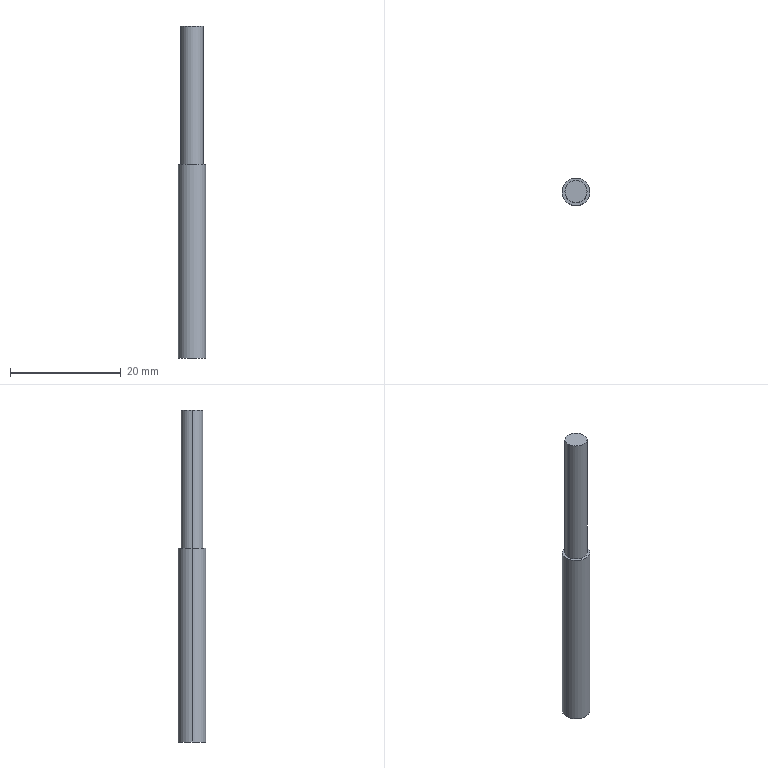Part | 1 solid | 7 faces | box 5 x 5 x 60 mm | volume 1001 mm3 | cylinder 4 | plane 3 | commonest cylinder face diameters 4 x2 5 x2
STEP:
#1=CARTESIAN_POINT('',(2.,0.,35.));
#2=VERTEX_POINT('',#1);
#3=CARTESIAN_POINT('',(-2.,0.,35.));
#4=VERTEX_POINT('',#3);
#5=CARTESIAN_POINT('',(0.,0.,35.));
#6=DIRECTION('',(0.,0.,1.));
#7=DIRECTION('',(1.,0.,0.));
#8=AXIS2_PLACEMENT_3D('',#5,#6,#7);
#9=CIRCLE('',#8,2.);
#10=EDGE_CURVE('',#2,#4,#9,.T.);
#11=ORIENTED_EDGE('',*,*,#10,.T.);
#12=CARTESIAN_POINT('',(-2.,0.,60.));
#13=VERTEX_POINT('',#12);
#14=CARTESIAN_POINT('',(-2.,0.,35.));
#15=DIRECTION('',(0.,0.,1.));
#16=VECTOR('',#15,1000.);
#17=LINE('',#14,#16);
#18=EDGE_CURVE('',#4,#13,#17,.T.);
#19=ORIENTED_EDGE('',*,*,#18,.T.);
#20=CARTESIAN_POINT('',(2.,0.,60.));
#21=VERTEX_POINT('',#20);
#22=CARTESIAN_POINT('',(0.,0.,60.));
#23=DIRECTION('',(0.,0.,1.));
#24=DIRECTION('',(1.,0.,0.));
#25=AXIS2_PLACEMENT_3D('',#22,#23,#24);
#26=CIRCLE('',#25,2.);
#27=EDGE_CURVE('',#21,#13,#26,.T.);
#28=ORIENTED_EDGE('',*,*,#27,.F.);
#29=CARTESIAN_POINT('',(2.,0.,35.));
#30=DIRECTION('',(0.,0.,1.));
#31=VECTOR('',#30,1000.);
#32=LINE('',#29,#31);
#33=EDGE_CURVE('',#2,#21,#32,.T.);
#34=ORIENTED_EDGE('',*,*,#33,.F.);
#35=EDGE_LOOP('',(#11,#19,#28,#34));
#36=FACE_OUTER_BOUND('',#35,.T.);
#37=CARTESIAN_POINT('',(0.,0.,35.));
#38=DIRECTION('',(0.,0.,1.));
#39=DIRECTION('',(1.,0.,0.));
#40=AXIS2_PLACEMENT_3D('',#37,#38,#39);
#41=CYLINDRICAL_SURFACE('',#40,2.);
#42=ADVANCED_FACE('',(#36),#41,.T.);
#43=CARTESIAN_POINT('',(2.5,0.,35.));
#44=VERTEX_POINT('',#43);
#45=CARTESIAN_POINT('',(-2.5,0.,35.));
#46=VERTEX_POINT('',#45);
#47=CARTESIAN_POINT('',(0.,0.,35.));
#48=DIRECTION('',(0.,0.,1.));
#49=DIRECTION('',(1.,0.,0.));
#50=AXIS2_PLACEMENT_3D('',#47,#48,#49);
#51=CIRCLE('',#50,2.5);
#52=EDGE_CURVE('',#44,#46,#51,.T.);
#53=ORIENTED_EDGE('',*,*,#52,.F.);
#54=CARTESIAN_POINT('',(2.5,0.,0.));
#55=VERTEX_POINT('',#54);
#56=CARTESIAN_POINT('',(2.5,0.,60.));
#57=DIRECTION('',(0.,0.,-1.));
#58=VECTOR('',#57,1000.);
#59=LINE('',#56,#58);
#60=EDGE_CURVE('',#44,#55,#59,.T.);
#61=ORIENTED_EDGE('',*,*,#60,.T.);
#62=CARTESIAN_POINT('',(-2.5,0.,0.));
#63=VERTEX_POINT('',#62);
#64=CARTESIAN_POINT('',(0.,0.,0.));
#65=DIRECTION('',(0.,0.,1.));
#66=DIRECTION('',(1.,0.,0.));
#67=AXIS2_PLACEMENT_3D('',#64,#65,#66);
#68=CIRCLE('',#67,2.5);
#69=EDGE_CURVE('',#55,#63,#68,.T.);
#70=ORIENTED_EDGE('',*,*,#69,.T.);
#71=CARTESIAN_POINT('',(-2.5,0.,60.));
#72=DIRECTION('',(0.,0.,-1.));
#73=VECTOR('',#72,1000.);
#74=LINE('',#71,#73);
#75=EDGE_CURVE('',#46,#63,#74,.T.);
#76=ORIENTED_EDGE('',*,*,#75,.F.);
#77=EDGE_LOOP('',(#53,#61,#70,#76));
#78=FACE_OUTER_BOUND('',#77,.T.);
#79=CARTESIAN_POINT('',(0.,0.,60.));
#80=DIRECTION('',(0.,0.,-1.));
#81=DIRECTION('',(-1.,0.,0.));
#82=AXIS2_PLACEMENT_3D('',#79,#80,#81);
#83=CYLINDRICAL_SURFACE('',#82,2.5);
#84=ADVANCED_FACE('',(#78),#83,.T.);
#85=ORIENTED_EDGE('',*,*,#60,.F.);
#86=CARTESIAN_POINT('',(0.,0.,35.));
#87=DIRECTION('',(0.,0.,1.));
#88=DIRECTION('',(1.,0.,0.));
#89=AXIS2_PLACEMENT_3D('',#86,#87,#88);
#90=CIRCLE('',#89,2.5);
#91=EDGE_CURVE('',#46,#44,#90,.T.);
#92=ORIENTED_EDGE('',*,*,#91,.F.);
#93=ORIENTED_EDGE('',*,*,#75,.T.);
#94=CARTESIAN_POINT('',(0.,0.,0.));
#95=DIRECTION('',(0.,0.,1.));
#96=DIRECTION('',(1.,0.,0.));
#97=AXIS2_PLACEMENT_3D('',#94,#95,#96);
#98=CIRCLE('',#97,2.5);
#99=EDGE_CURVE('',#63,#55,#98,.T.);
#100=ORIENTED_EDGE('',*,*,#99,.T.);
#101=EDGE_LOOP('',(#85,#92,#93,#100));
#102=FACE_OUTER_BOUND('',#101,.T.);
#103=CARTESIAN_POINT('',(0.,0.,60.));
#104=DIRECTION('',(0.,0.,-1.));
#105=DIRECTION('',(-1.,0.,0.));
#106=AXIS2_PLACEMENT_3D('',#103,#104,#105);
#107=CYLINDRICAL_SURFACE('',#106,2.5);
#108=ADVANCED_FACE('',(#102),#107,.T.);
#109=ORIENTED_EDGE('',*,*,#99,.F.);
#110=ORIENTED_EDGE('',*,*,#69,.F.);
#111=EDGE_LOOP('',(#109,#110));
#112=FACE_OUTER_BOUND('',#111,.T.);
#113=CARTESIAN_POINT('',(0.,0.,0.));
#114=DIRECTION('',(0.,0.,1.));
#115=DIRECTION('',(1.,0.,0.));
#116=AXIS2_PLACEMENT_3D('',#113,#114,#115);
#117=PLANE('',#116);
#118=ADVANCED_FACE('',(#112),#117,.F.);
#119=ORIENTED_EDGE('',*,*,#10,.F.);
#120=CARTESIAN_POINT('',(0.,0.,35.));
#121=DIRECTION('',(0.,0.,1.));
#122=DIRECTION('',(1.,0.,0.));
#123=AXIS2_PLACEMENT_3D('',#120,#121,#122);
#124=CIRCLE('',#123,2.);
#125=EDGE_CURVE('',#4,#2,#124,.T.);
#126=ORIENTED_EDGE('',*,*,#125,.F.);
#127=EDGE_LOOP('',(#119,#126));
#128=FACE_BOUND('',#127,.T.);
#129=ORIENTED_EDGE('',*,*,#91,.T.);
#130=ORIENTED_EDGE('',*,*,#52,.T.);
#131=EDGE_LOOP('',(#129,#130));
#132=FACE_OUTER_BOUND('',#131,.T.);
#133=CARTESIAN_POINT('',(0.,0.,35.));
#134=DIRECTION('',(0.,0.,1.));
#135=DIRECTION('',(1.,0.,0.));
#136=AXIS2_PLACEMENT_3D('',#133,#134,#135);
#137=PLANE('',#136);
#138=ADVANCED_FACE('',(#128,#132),#137,.T.);
#139=ORIENTED_EDGE('',*,*,#18,.F.);
#140=ORIENTED_EDGE('',*,*,#125,.T.);
#141=ORIENTED_EDGE('',*,*,#33,.T.);
#142=CARTESIAN_POINT('',(0.,0.,60.));
#143=DIRECTION('',(0.,0.,1.));
#144=DIRECTION('',(1.,0.,0.));
#145=AXIS2_PLACEMENT_3D('',#142,#143,#144);
#146=CIRCLE('',#145,2.);
#147=EDGE_CURVE('',#13,#21,#146,.T.);
#148=ORIENTED_EDGE('',*,*,#147,.F.);
#149=EDGE_LOOP('',(#139,#140,#141,#148));
#150=FACE_OUTER_BOUND('',#149,.T.);
#151=CARTESIAN_POINT('',(0.,0.,35.));
#152=DIRECTION('',(0.,0.,1.));
#153=DIRECTION('',(1.,0.,0.));
#154=AXIS2_PLACEMENT_3D('',#151,#152,#153);
#155=CYLINDRICAL_SURFACE('',#154,2.);
#156=ADVANCED_FACE('',(#150),#155,.T.);
#157=ORIENTED_EDGE('',*,*,#27,.T.);
#158=ORIENTED_EDGE('',*,*,#147,.T.);
#159=EDGE_LOOP('',(#157,#158));
#160=FACE_OUTER_BOUND('',#159,.T.);
#161=CARTESIAN_POINT('',(0.,0.,60.));
#162=DIRECTION('',(0.,0.,1.));
#163=DIRECTION('',(1.,0.,0.));
#164=AXIS2_PLACEMENT_3D('',#161,#162,#163);
#165=PLANE('',#164);
#166=ADVANCED_FACE('',(#160),#165,.T.);
#167=CLOSED_SHELL('',(#42,#84,#108,#118,#138,#156,#166));
#168=MANIFOLD_SOLID_BREP('',#167);
#169=CARTESIAN_POINT('',(0.,0.,0.));
#170=DIRECTION('',(0.,0.,1.));
#171=DIRECTION('',(1.,0.,0.));
#172=AXIS2_PLACEMENT_3D('',#169,#170,#171);
#173=(LENGTH_UNIT()NAMED_UNIT(*)SI_UNIT(.MILLI.,.METRE.));
#174=UNCERTAINTY_MEASURE_WITH_UNIT(LENGTH_MEASURE(0.00001),#173,'','');
#175=(NAMED_UNIT(*)PLANE_ANGLE_UNIT()SI_UNIT($,.RADIAN.));
#176=(NAMED_UNIT(*)SI_UNIT($,.STERADIAN.)SOLID_ANGLE_UNIT());
#177=(GEOMETRIC_REPRESENTATION_CONTEXT(3)GLOBAL_UNCERTAINTY_ASSIGNED_CONTEXT((#174))GLOBAL_UNIT_ASSIGNED_CONTEXT((#173,#175,#176))REPRESENTATION_CONTEXT('',''));
#178=ADVANCED_BREP_SHAPE_REPRESENTATION('',(#168,#172),#177);